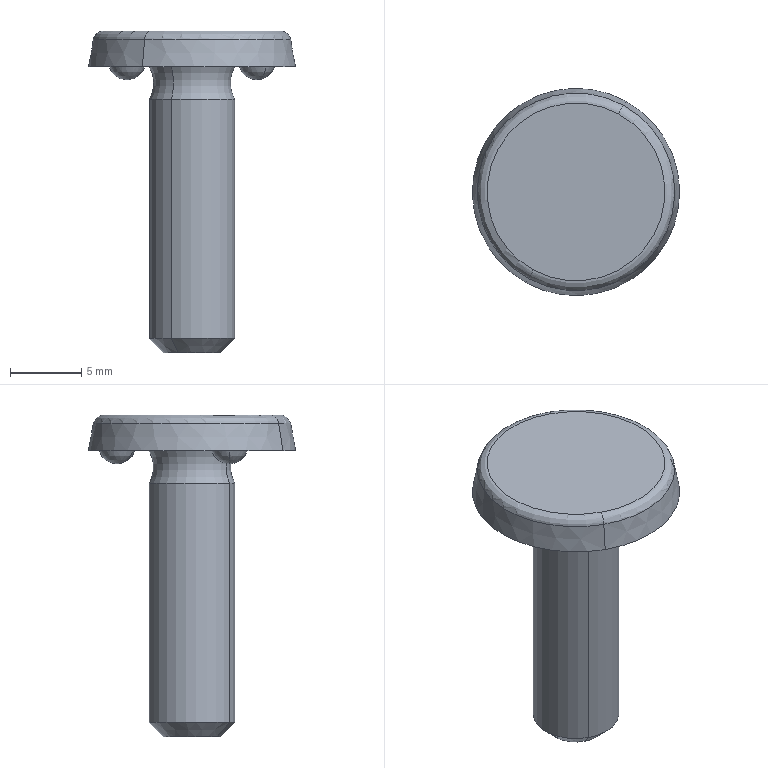Part | 1 solid | 19 faces | box 14.5 x 14.5 x 22.5 mm | volume 941.772 mm3 | sphere 6 | cone 4 | torus 4 | plane 3 | cylinder 2 | commonest cylinder face diameters 6 x2